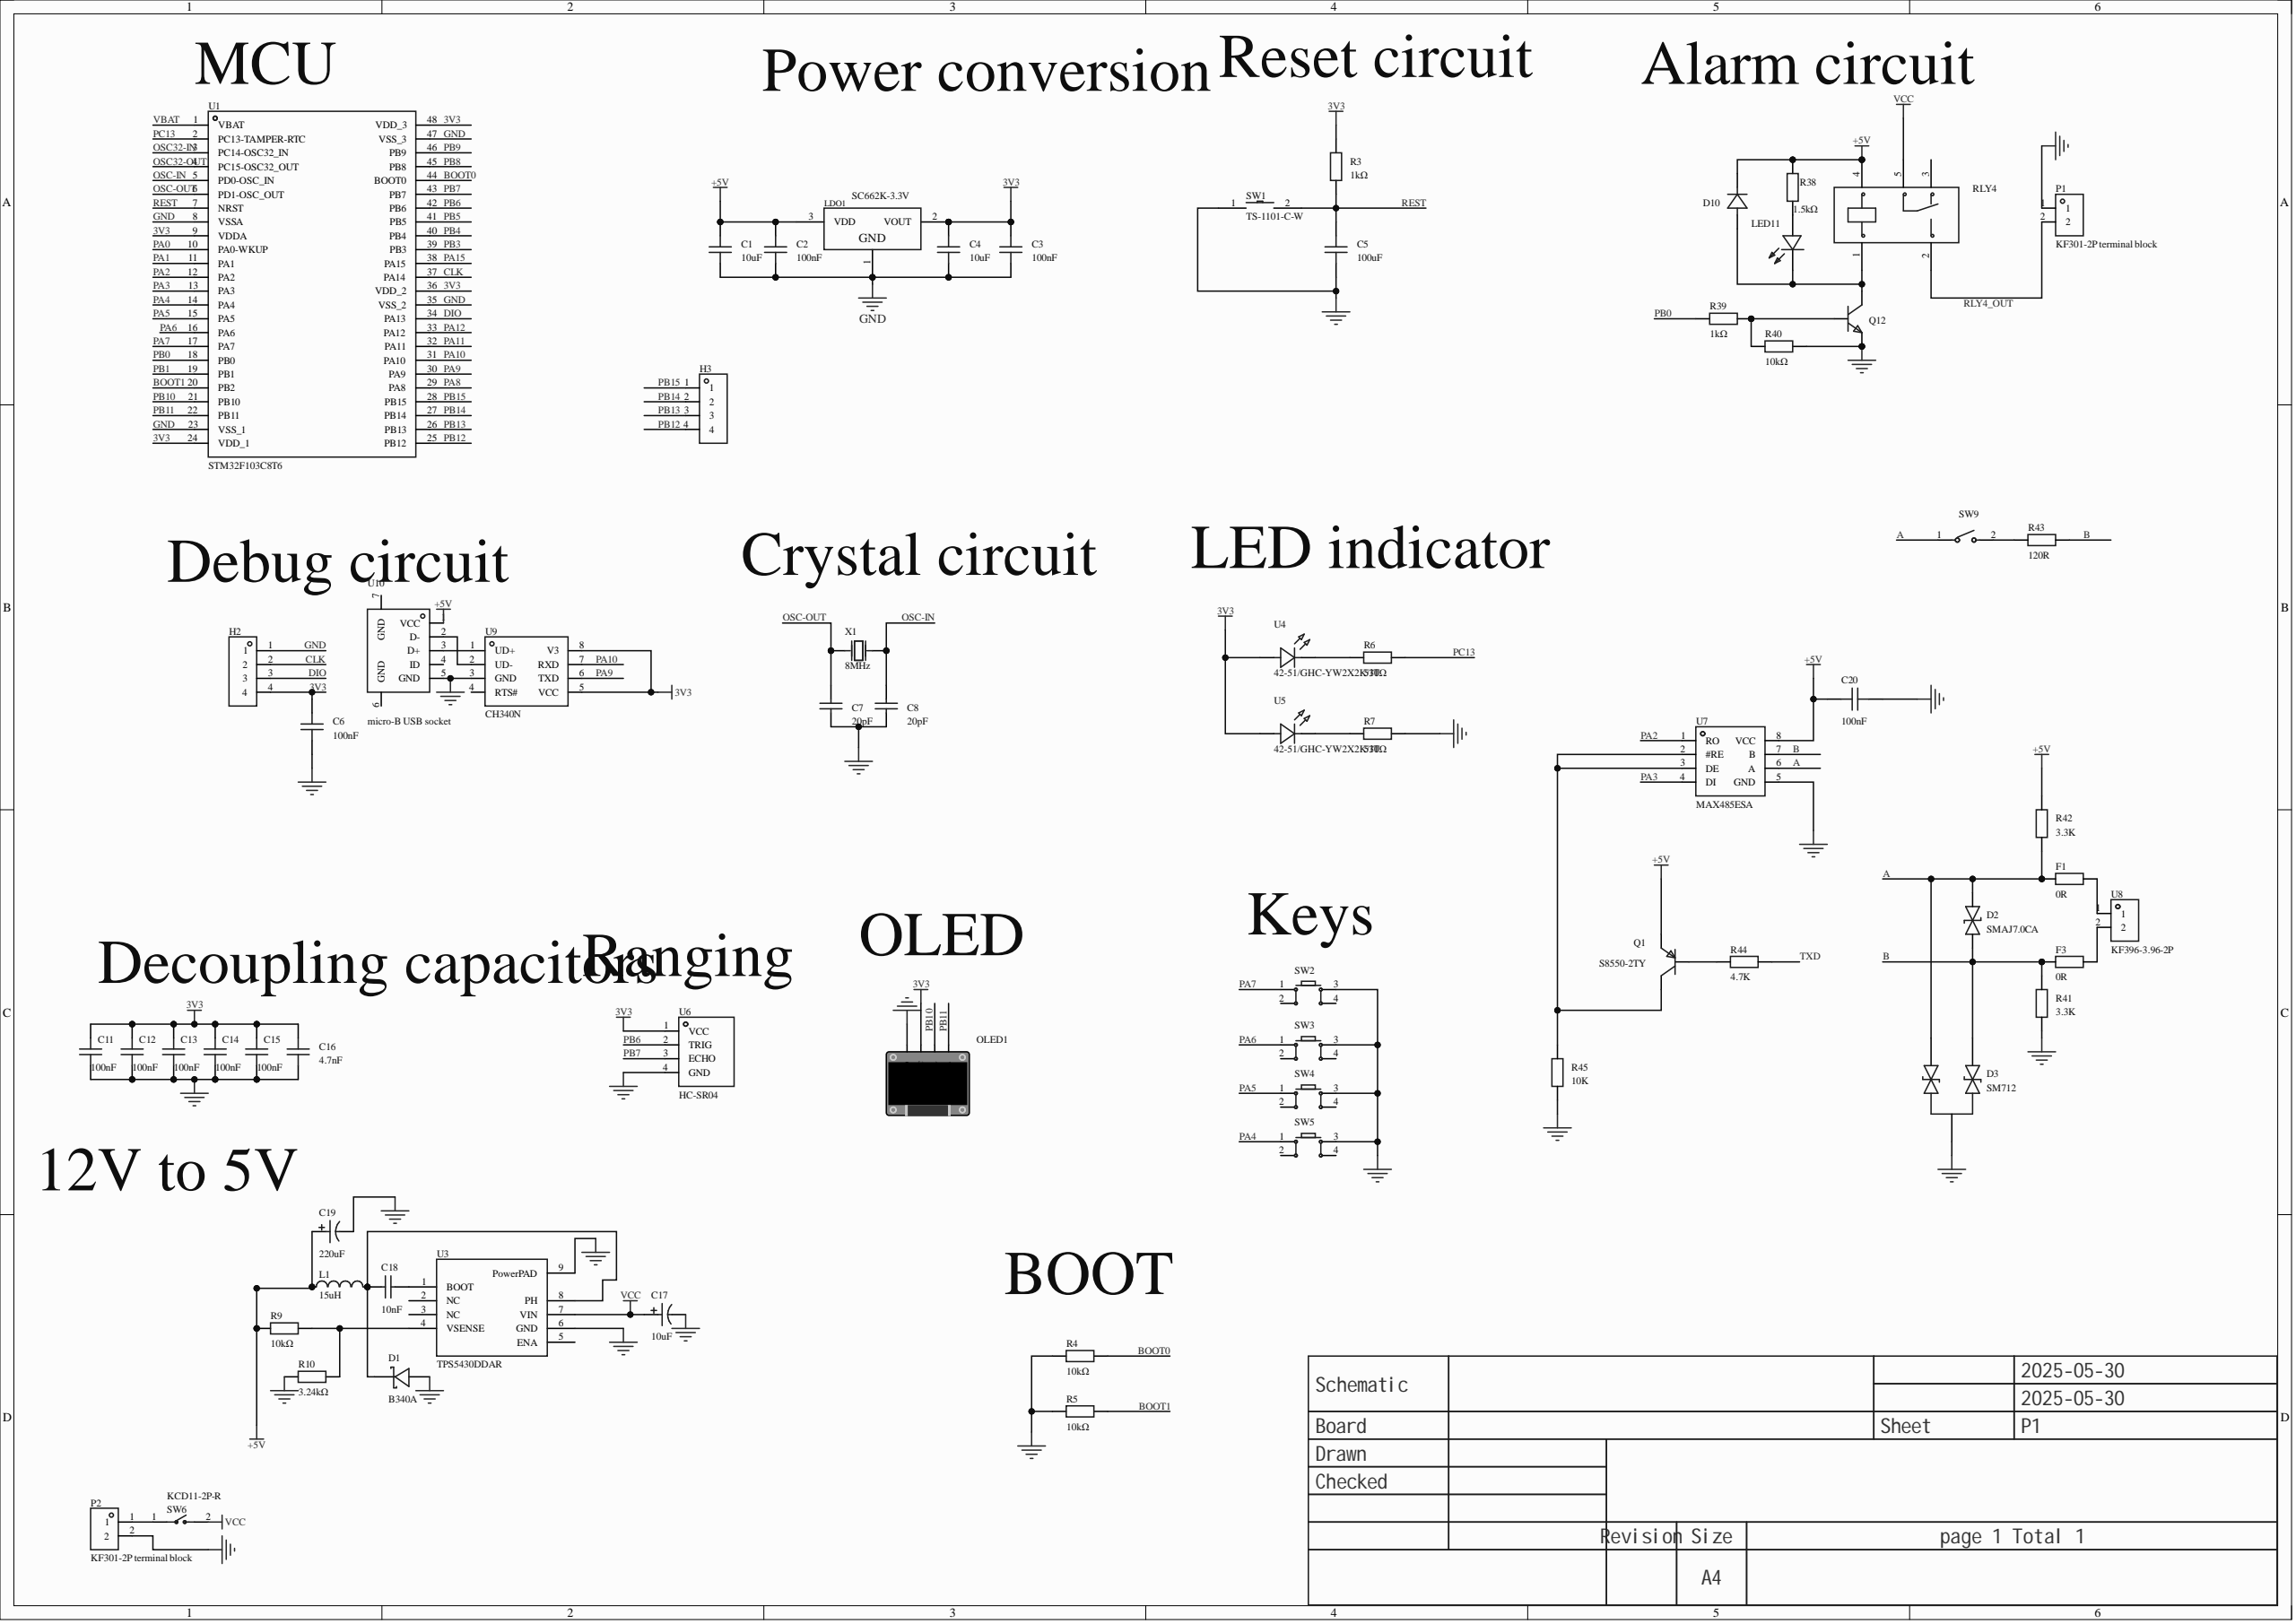Circuit board | Altium Designer | 67 parts | 48 nets
Bill of materials:
Comment,Description,Designator,Footprint,LibRef,Quantity
"10uF","Capacitance:10uF;Tolerance:±10%;Rated voltage:10V;Dielectric (temp. coefficient):X5R;","C1, C4","C0603","CL10A106KP8NNNC","2"
"100nF","Capacitance:100nF;Tolerance:±10%;Rated voltage:50V;Dielectric (temp. coefficient):X7R;, [NoValue]","C2, C3, C6, C11, C12, C13, C14, C15, C20","C0603","CC0603KRX7R9BB104, CGA0603X7R104K500JT, CAP_0603","9"
"100uF","Capacitance:100uF;Tolerance:±20%;Rated voltage:10V;Dielectric (temp. coefficient):X5R;","C5","C1206","HGC1206R5107M100NSPJ","1"
"20pF","Capacitance:20pF;Tolerance:±5%;Rated voltage:50V;Dielectric (temp. coefficient):C0G;","C7, C8","C0603","CL10C200JB8NNNC","2"
"4.7nF","Capacitance:4.7nF;Tolerance:±10%;Rated voltage:50V;Dielectric (temp. coefficient):X7R;","C16","C0603","CGA0603X7R472K500JT","1"
"10uF","Capacitance:10uF;Tolerance:±20%;Rated voltage:50V;","C17","CAP-TH_BD5.0-P2.00-D0.8-FD","KM106M050D11RR0VH2FP0","1"
"10nF","Capacitance:10nF;Tolerance:±10%;Rated voltage:50V;Dielectric (temp. coefficient):X7R;","C18","C0603","CC0603KRX7R9BB103","1"
"220uF","Capacitance:220uF;Tolerance:±20%;Rated voltage:16V;Ripple current:-;Equivalent series resistance:-;","C19","CAP-TH_BD6.3-P2.50-D1.0-FD","KM227M016E11RR0VH2FP0","1"
"B340A","Forward voltage drop (Vf):550mV@3A;DC reverse voltage (Vr):40V;Average rectified current (Io):3A;","D1","SMA_L4.3-W2.6-LS5.1-RD","B340A","1"
"SMAJ7.0CA","Reverse standoff voltage (Vrwm):7V;Max clamping voltage:12V;Peak pulse current (Ipp)@10/1000us:33.3A;Breakdown voltage:7.78V;","D2","SMA_L4.5-W2.7-LS5.1-BI","SMAJ7.0CA_C383701","1"
"SM712","","D3","SOT-23-3_L2.9-W1.3-P1.90-LS2.4-BR","SM712_C521963","1"
"1N4007","Diode configuration:Single;Forward voltage drop (Vf):1.1V@1A;DC reverse voltage (Vr):1kV;Rectified current:1A;","D10","SMA_L4.3-W2.5-LS5.0-RD","1N4007_C727081","1"
"0R","","F1, F3","R0805","Res_0805","2"
"","","H2, H3","HDR-TH_4P-P2.54-V-M","HDR-M_2.54_1x4P","2"
"15uH","Inductance:15uH;Tolerance:±20%;Rated current:3A;Saturation current (Isat):4.5A;Type:Integrally molded inductor;","L1","IND-SMD_L7.0-W6.6_FXL0630","FXL0630-150-M","1"
"SC662K-3.3V","Output type:Fixed;Output polarity:Positive;Max input voltage:6V;Output voltage:3.3V;Output current:250mA;Power supply ripple rejection (PSRR):50dB@(1kHz);","LDO1","SOT-23-3_L2.9-W1.3-P1.90-LS2.4-BR","SC662K-3.3V","1"
"NCD0805R1","灯头类型:-;发光颜色:红色;正向电压(VF):1.6V~2.6V;功率:65mW;正向电流:20mA;主波长:615nm~630nm;二极管配置:独立二极管;透镜颜色:无色透明透镜;色温:-;发光强度:67mcd~195mcd;发光角度:130°;载带方式:-;工作温度:-30℃~+85℃;","LED11","LED0805-R-RD","NCD0805R1","1"
"","","OLED1","0.96OLED_4P","0.96OLED模块_4P","1"
"KF301-2P terminal block","","P1, P2","CONN-TH_XY301V-A-5.0-2P","KF301-2P接线端子","2"
"S8550-2TY","Transistor type:PNP;Collector current (Ic):1.5A;Collector-emitter breakdown voltage (Vceo):25V;Power (Pd):300mW;","Q1","SOT-23-3_L2.9-W1.3-P0.95-LS2.4-BR","S8550-2TY","1"
"S8050 J3Y(RANGE:200-350)","Transistor type:NPN;Collector current (Ic):500mA;Collector-emitter breakdown voltage (Vceo):25V;Power dissipation (Pd):300mW;DC current gain (hFE):200@500mA,1V;","Q12","SOT-23-3_L3.0-W1.7-P0.95-LS2.9-BR","S8050 J3Y(RANGE:200-350)","1"
"1kΩ","Resistor type:Thick-film resistor;Resistance:1kΩ;Tolerance:±1%;Power:100mW;Max working voltage:75V;Temperature coefficient:±100ppm/?;","R3","R0603","RC0603FR-071KL","1"
"10kΩ","Resistor type:Thick-film resistor;Resistance:10kΩ;Tolerance:±1%;Power:100mW;Max working voltage:75V;Temperature coefficient:±100ppm/?;","R4, R5, R9","R0603","0603WAF1002T5E","3"
"510Ω","Resistor type:Thick-film resistor;Resistance:510Ω;Tolerance:±1%;Power:100mW;Max working voltage:75V;Temperature coefficient:±100ppm/?;","R6, R7","R0603","0603WAF5100T5E","2"
"3.24kΩ","Resistor type:Thick-film resistor;Resistance:3.24kΩ;Tolerance:±1%;Power:100mW;Max working voltage:75V;Temperature coefficient:±100ppm/?;","R10","R0603","0603WAF3241T5E","1"
"1.5kΩ","Resistor type:Thick-film resistor;Resistance:1.5kΩ;Tolerance:±1%;Power:125mW;Max working voltage:150V;Temperature coefficient:±100ppm/?;","R38","R0805","0805W8F1501T5E","1"
"1kΩ","Resistor type:Thick-film resistor;Resistance:1kΩ;Tolerance:±1%;Power:125mW;Max working voltage:150V;Temperature coefficient:±100ppm/?;","R39","R0805","0805W8F1001T5E","1"
"10kΩ","Resistor type:Thick-film resistor;Resistance:10kΩ;Tolerance:±1%;Power:125mW;Max working voltage:150V;Temperature coefficient:±100ppm/?;","R40","R0805","0805W8F1002T5E_C17414","1"
"3.3K","","R41, R42","R0603","Res_0603","2"
"120R","","R43","R0603","Res_0603","1"
"4.7K","","R44","R0603","Res_0603","1"
"10K","","R45","R0603","Res_0603","1"
"SRD-05VDC-SL-C","Coil voltage:5V;Contact form:1C (SPDT changeover);Contact rating (resistive load):-;Max switching voltage:250V@AC;Max switching current:15A;","RLY4","RELAY-TH_SRD-XXVDC-XL-C","SRD-05VDC-SL-C","1"
"TS-1101-C-W","电路结构:单刀单掷;按钮形状:矩形按钮;作用力:260gf;安装方式:立贴;开关长度:6mm;开关宽度:3.6mm;开关高度:2.5mm;带支架:不带;触点电流:50mA;额定电压(AC):-;额定电压(DC):12V;额定功率:-;绝缘电阻:-;带灯:无;机械寿命:5万次;","SW1","SW-SMD_L6.0-W3.3-LS8.0","TS-1101-C-W","1"
"","","SW2, SW3, SW4, SW5","SW-TH_4P-L6.0-W6.0-P4.50-LS6.5","Key_TH_6x6x6","4"
"KCD11-2P-R","Lamp:None;Pin style:Solder tab;Rated current:3A;Rated voltage (AC):250V;Rated voltage (DC):-;Circuit structure:SPST;Mechanical life:1万 cycles;","SW6","SW-TH_2P-L15.0-W10.5-P5.00_KCD11-2P-R","KCD11-2P-R","1"
"ZX-1.27BM-1PSMD","Type:Slide, recessed;Circuit structure:SPST;Number of positions:1;Rated current:25mA;Rated voltage:24V;Service life:1千 cycles;Color:Black;","SW9","SW-SMD_L5.4-W2.8-LS8.2","ZX-1.27BM-1PSMD","1"
"STM32F103C8T6","CPU内核:ARM-M3;程序存储容量:64KB;RAM总容量:20KB;GPIO端口数量:37;工作电压范围:2V~3.6V;CPU最大主频:72MHz;程序存储器类型:FLASH;","U1","LQFP-48_L7.0-W7.0-P0.50-LS9.0-BL","STM32F103C8T6","1"
"TPS5430DDAR","Function type:Step-down;Output type:Adjustable;Input voltage:5.5V~36V;Output voltage:1.221V~32.04V;Output current (max):3A;","U3","ESOP-8_L4.9-W3.9-P1.27-LS6.0-TL-EP","TPS5430DDAR","1"
"42-51/GHC-YW2X2K/3T","Emitted color:Emerald green;Forward current:-;Dominant wavelength:520nm~535nm;Luminous intensity:2850mcd;","U4, U5","LED-SMD_L1.6-W0.8-FD_GREEN-1","42-51/GHC-YW2X2K/3T","2"
"HC-SR04","","U6","TH_HC-SR04V","HC-SR04","1"
"MAX485ESA","","U7","SOP-8_L5.0-W4.0-P1.27-LS6.0-BL","MAX485ESA_C668206","1"
"KF396-3.96-2P","结构:1x2P;间距:3.96mm;颜色:绿色;安装方式:直插;额定电流:10A;额定电压:300V;排数:1;线规 - AWG:18~24;线规 - 平方毫米:0.75;每排PIN数:2;工作温度范围:-40℃~+105℃;","U8","CONN-TH_P3.96_KF396-3.96-2P","KF396-3.96-2P","1"
"CH340N","Application function:USB-to-serial;Interface protocol:USB 2.0;Channels:1;Data rate:2Mbps;","U9","SOP-8_L4.9-W3.9-P1.27-LS6.0-BL","CH340N","1"
"micro-B USB socket","","U10","MICRO-USB_C9900039549","micro-b usb母座","1"
"8MHz","Crystal type:Through-hole crystal;Frequency:8MHz;Frequency deviation at room temp:±20ppm;External load capacitance:20pF;Frequency stability (full temp):±30ppm;","X1","OSC-TH_L10.0-W4.5-P5.00","X49SD8MSD2SC","1"
Netlist (Protel format):
[
C1
C0603
10uF



]
[
C2
C0603
100nF



]
[
C3
C0603
100nF



]
[
C4
C0603
10uF



]
[
C5
C1206
100uF



]
[
C6
C0603
100nF



]
[
C7
C0603
20pF



]
[
C8
C0603
20pF



]
[
C11
C0603
100nF



]
[
C12
C0603
100nF



]
[
C13
C0603
100nF



]
[
C14
C0603
100nF



]
[
C15
C0603
100nF



]
[
C16
C0603
4.7nF



]
[
C17
CAP-TH_BD5.0-P2.00-D0.8-FD
10uF



]
[
C18
C0603
10nF



]
[
C19
CAP-TH_BD6.3-P2.50-D1.0-FD
220uF



]
[
C20
C0603
100nF



]
[
D1
SMA_L4.3-W2.6-LS5.1-RD
B340A



]
[
D2
SMA_L4.5-W2.7-LS5.1-BI
SMAJ7.0CA



]
[
D3
SOT-23-3_L2.9-W1.3-P1.90-LS2.4-BR
SM712



]
[
D10
SMA_L4.3-W2.5-LS5.0-RD
1N4007



]
[
F1
R0805
0R



]
[
F3
R0805
0R



]
[
H2
HDR-TH_4P-P2.54-V-M




]
[
H3
HDR-TH_4P-P2.54-V-M




]
[
L1
IND-SMD_L7.0-W6.6_FXL0630
15uH



]
[
LDO1
SOT-23-3_L2.9-W1.3-P1.90-LS2.4-BR
SC662K-3.3V



]
[
LED11
LED0805-R-RD
NCD0805R1



]
[
OLED1
0.96OLED_4P




]
[
P1
CONN-TH_XY301V-A-5.0-2P
KF301-2P terminal block



]
[
P2
CONN-TH_XY301V-A-5.0-2P
KF301-2P terminal block



]
[
Q1
SOT-23-3_L2.9-W1.3-P0.95-LS2.4-BR
S8550-2TY



]
[
Q12
SOT-23-3_L3.0-W1.7-P0.95-LS2.9-BR
S8050 J3Y(RANGE:200-350)



]
[
R3
R0603
1kΩ



]
[
R4
R0603
10kΩ



]
[
R5
R0603
10kΩ



]
[
R6
R0603
510Ω



]
[
R7
R0603
510Ω



]
[
R9
R0603
10kΩ



]
[
R10
R0603
3.24kΩ



]
[
R38
R0805
1.5kΩ



]
[
R39
R0805
1kΩ



]
[
R40
R0805
10kΩ



]
[
R41
R0603
3.3K



]
[
R42
R0603
3.3K



]
[
R43
R0603
120R



]
[
R44
R0603
4.7K



]
[
R45
R0603
10K



]
[
RLY4
RELAY-TH_SRD-XXVDC-XL-C
SRD-05VDC-SL-C



]
[
SW1
SW-SMD_L6.0-W3.3-LS8.0
TS-1101-C-W



]
[
SW2
SW-TH_4P-L6.0-W6.0-P4.50-LS6.5




]
[
SW3
SW-TH_4P-L6.0-W6.0-P4.50-LS6.5




]
[
SW4
SW-TH_4P-L6.0-W6.0-P4.50-LS6.5




]
[
SW5
SW-TH_4P-L6.0-W6.0-P4.50-LS6.5




]
[
SW6
SW-TH_2P-L15.0-W10.5-P5.00_KCD11-2P-R
KCD11-2P-R



]
[
SW9
SW-SMD_L5.4-W2.8-LS8.2
ZX-1.27BM-1PSMD



]
[
U1
LQFP-48_L7.0-W7.0-P0.50-LS9.0-BL
STM32F103C8T6



]
[
U3
ESOP-8_L4.9-W3.9-P1.27-LS6.0-TL-EP
TPS5430DDAR



]
[
U4
LED-SMD_L1.6-W0.8-FD_GREEN-1
42-51/GHC-YW2X2K/3T



]
[
U5
LED-SMD_L1.6-W0.8-FD_GREEN-1
42-51/GHC-YW2X2K/3T



]
[
U6
TH_HC-SR04V
HC-SR04



]
[
U7
SOP-8_L5.0-W4.0-P1.27-LS6.0-BL
MAX485ESA



]
[
U8
CONN-TH_P3.96_KF396-3.96-2P
KF396-3.96-2P



]
[
U9
SOP-8_L4.9-W3.9-P1.27-LS6.0-BL
CH340N



]
[
U10
MICRO-USB_C9900039549
micro-B USB socket



]
[
X1
OSC-TH_L10.0-W4.5-P5.00
8MHz



]
(
VCC
C17-1
RLY4-5
SW6-2
U3-7
)
(
RLY4_OUT
P1-2
RLY4-2
)
(
REST
C5-2
R3-1
SW1-2
U1-7
)
(
PC13
R6-2
U1-2
)
(
PB15
H3-1
U1-28
)
(
PB14
H3-2
U1-27
)
(
PB13
H3-3
U1-26
)
(
PB12
H3-4
U1-25
)
(
PB11
OLED1-4
U1-22
)
(
PB10
OLED1-3
U1-21
)
(
PB7
U1-43
U6-3
)
(
PB6
U1-42
U6-2
)
(
PB0
R39-1
U1-18
)
(
PA10
U1-31
U9-7
)
(
PA9
U1-30
U9-6
)
(
PA7
SW2-1
U1-17
)
(
PA6
SW3-1
U1-16
)
(
PA5
SW4-1
U1-15
)
(
PA4
SW5-1
U1-14
)
(
PA3
U1-13
U7-4
)
(
PA2
U1-12
U7-1
)
(
OSC-OUT
C7-2
U1-6
X1-2
)
(
OSC-IN
C8-2
U1-5
X1-1
)
(
NetU9_2
U9-2
U10-2
)
(
NetU9_1
U9-1
U10-3
)
(
NetR43_1
R43-1
SW9-2
)
(
NetR9_2
R9-2
R10-2
U3-4
)
(
NetR7_1
R7-1
U5-2
)
(
NetR6_1
R6-1
U4-2
)
(
NetQ12_1
Q12-1
R39-2
R40-2
)
(
NetQ1_3
Q1-3
R45-1
U7-2
U7-3
)
(
NetQ1_1
Q1-1
R44-2
)
(
NetP2_1
P2-1
SW6-1
)
(
NetLED11_1
LED11-1
R38-1
)
(
NetF3_2
F3-2
U8-2
)
(
NetF1_2
F1-2
U8-1
)
(
NetD10_2
D10-2
LED11-2
Q12-3
RLY4-1
)
(
NetC18_2
C18-2
U3-1
)
(
NetC18_1
C18-1
D1-1
L1-2
U3-8
)
(
GND
C1-1
C2-1
C3-1
C4-1
C5-1
C6-1
C7-1
C8-1
C11-1
C12-1
C13-1
C14-1
C15-1
C16-1
C17-2
C19-2
C20-2
D1-2
D3-3
H2-1
LDO1-1
OLED1-1
P1-1
P2-2
Q12-2
R4-1
R5-1
R7-2
R10-1
R40-1
R41-1
R45-2
SW1-1
SW2-3
SW3-3
SW4-3
SW5-3
U1-8
U1-23
U1-35
U1-47
U3-6
U3-9
U6-4
U7-5
U9-3
U10-5
)
(
DIO
H2-3
U1-34
)
(
CLK
H2-2
U1-37
)
(
BOOT1
R5-2
U1-20
)
(
BOOT0
R4-2
U1-44
)
(
B
D2-1
D3-1
F3-1
R41-2
R43-2
U7-7
)
(
A
D2-2
D3-2
F1-1
R42-1
SW9-1
U7-6
)
(
+5V
C1-2
C2-2
C19-1
C20-1
D10-1
L1-1
LDO1-3
Q1-2
R9-1
R38-2
R42-2
RLY4-4
U7-8
U10-1
)
(
3V3
C3-2
C4-2
C6-2
C11-2
C12-2
C13-2
C14-2
C15-2
C16-2
H2-4
LDO1-2
OLED1-2
R3-2
U1-9
U1-24
U1-36
U1-48
U4-1
U5-1
U6-1
U9-5
U9-8
)